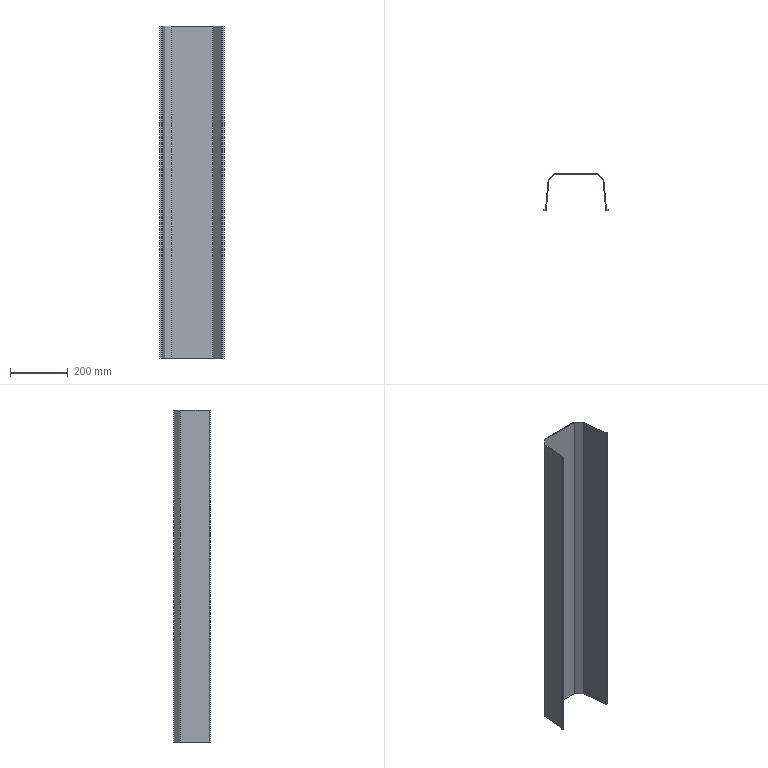Part | STEP file | 51E-01223JG10 | 1 solid | 56 faces | box 225 x 127 x 1150 mm | volume 1231792 mm3 | plane 40 | cylinder 16 | commonest cylinder face diameters 2 x6 7 x6 2.5 x4
STEP:
#1=CARTESIAN_POINT('',(-106.207,0.,575.));
#2=VERTEX_POINT('',#1);
#3=CARTESIAN_POINT('',(-106.207,2.5,575.));
#4=VERTEX_POINT('',#3);
#5=CARTESIAN_POINT('',(-106.207,1.25,575.));
#6=DIRECTION('',(0.,1.,0.));
#7=VECTOR('',#6,1.);
#8=LINE('',#5,#7);
#9=EDGE_CURVE('',#2,#4,#8,.T.);
#10=ORIENTED_EDGE('',*,*,#9,.F.);
#11=CARTESIAN_POINT('',(-102.72,3.195,575.));
#12=VERTEX_POINT('',#11);
#13=CARTESIAN_POINT('',(-102.72,3.195,575.));
#14=CARTESIAN_POINT('',(-102.752,2.83,575.));
#15=CARTESIAN_POINT('',(-102.832,2.469,575.));
#16=CARTESIAN_POINT('',(-102.959,2.12,575.));
#17=CARTESIAN_POINT('',(-103.301,1.465,575.));
#18=CARTESIAN_POINT('',(-103.8,0.9191,575.));
#19=CARTESIAN_POINT('',(-104.084,0.6808,575.));
#20=CARTESIAN_POINT('',(-104.656,0.3172,575.));
#21=CARTESIAN_POINT('',(-105.296,0.09984,575.));
#22=CARTESIAN_POINT('',(-105.597,0.03328,575.));
#23=CARTESIAN_POINT('',(-105.902,0.,575.));
#24=CARTESIAN_POINT('',(-106.207,0.,575.));
#25=B_SPLINE_CURVE_WITH_KNOTS('',5,(#13,#14,#15,#16,#17,#18,#19,#20,#21,#22,#23,#24),.UNSPECIFIED.,.F.,.U.,(6,3,3,6),(0.,2.592,5.185,7.343),.UNSPECIFIED.);
#26=EDGE_CURVE('',#12,#2,#25,.T.);
#27=ORIENTED_EDGE('',*,*,#26,.F.);
#28=CARTESIAN_POINT('',(-105.211,3.413,575.));
#29=VERTEX_POINT('',#28);
#30=CARTESIAN_POINT('',(-103.966,3.304,575.));
#31=DIRECTION('',(0.9962,-0.08716,0.));
#32=VECTOR('',#31,1.);
#33=LINE('',#30,#32);
#34=EDGE_CURVE('',#29,#12,#33,.T.);
#35=ORIENTED_EDGE('',*,*,#34,.F.);
#36=CARTESIAN_POINT('',(-105.211,3.413,575.));
#37=CARTESIAN_POINT('',(-105.22,3.315,575.));
#38=CARTESIAN_POINT('',(-105.24,3.219,575.));
#39=CARTESIAN_POINT('',(-105.272,3.125,575.));
#40=CARTESIAN_POINT('',(-105.359,2.948,575.));
#41=CARTESIAN_POINT('',(-105.486,2.797,575.));
#42=CARTESIAN_POINT('',(-105.559,2.729,575.));
#43=CARTESIAN_POINT('',(-105.719,2.614,575.));
#44=CARTESIAN_POINT('',(-105.902,2.54,575.));
#45=CARTESIAN_POINT('',(-105.998,2.515,575.));
#46=CARTESIAN_POINT('',(-106.098,2.501,575.));
#47=CARTESIAN_POINT('',(-106.199,2.5,575.));
#48=CARTESIAN_POINT('',(-106.202,2.5,575.));
#49=CARTESIAN_POINT('',(-106.204,2.5,575.));
#50=CARTESIAN_POINT('',(-106.207,2.5,575.));
#51=B_SPLINE_CURVE_WITH_KNOTS('',5,(#36,#37,#38,#39,#40,#41,#42,#43,#44,#45,#46,#47,#48,#49,#50),.UNSPECIFIED.,.F.,.U.,(6,3,3,3,6),(0.,0.6928,1.386,2.078,2.098),.UNSPECIFIED.);
#52=EDGE_CURVE('',#29,#4,#51,.T.);
#53=ORIENTED_EDGE('',*,*,#52,.T.);
#54=EDGE_LOOP('',(#10,#27,#35,#53));
#55=FACE_OUTER_BOUND('',#54,.T.);
#56=CARTESIAN_POINT('',(-106.207,0.,575.));
#57=DIRECTION('',(0.,0.,1.));
#58=DIRECTION('',(1.,0.,0.));
#59=AXIS2_PLACEMENT_3D('',#56,#57,#58);
#60=PLANE('',#59);
#61=ADVANCED_FACE('',(#55),#60,.T.);
#62=CARTESIAN_POINT('',(-111.25,2.5,575.));
#63=VERTEX_POINT('',#62);
#64=CARTESIAN_POINT('',(-112.5,1.25,575.));
#65=VERTEX_POINT('',#64);
#66=CARTESIAN_POINT('',(-111.25,1.25,575.));
#67=DIRECTION('',(0.,0.,1.));
#68=AXIS2_PLACEMENT_3D('',#66,#67,$);
#69=CIRCLE('',#68,1.25);
#70=EDGE_CURVE('',#63,#65,#69,.T.);
#71=ORIENTED_EDGE('',*,*,#70,.T.);
#72=CARTESIAN_POINT('',(-111.25,0.,575.));
#73=VERTEX_POINT('',#72);
#74=CARTESIAN_POINT('',(-111.25,1.25,575.));
#75=DIRECTION('',(0.,0.,1.));
#76=AXIS2_PLACEMENT_3D('',#74,#75,$);
#77=CIRCLE('',#76,1.25);
#78=EDGE_CURVE('',#65,#73,#77,.T.);
#79=ORIENTED_EDGE('',*,*,#78,.T.);
#80=CARTESIAN_POINT('',(-108.729,0.,575.));
#81=DIRECTION('',(-1.,0.,0.));
#82=VECTOR('',#81,1.);
#83=LINE('',#80,#82);
#84=EDGE_CURVE('',#2,#73,#83,.T.);
#85=ORIENTED_EDGE('',*,*,#84,.F.);
#86=ORIENTED_EDGE('',*,*,#9,.T.);
#87=CARTESIAN_POINT('',(-108.729,2.5,575.));
#88=DIRECTION('',(-1.,0.,0.));
#89=VECTOR('',#88,1.);
#90=LINE('',#87,#89);
#91=EDGE_CURVE('',#4,#63,#90,.T.);
#92=ORIENTED_EDGE('',*,*,#91,.T.);
#93=EDGE_LOOP('',(#71,#79,#85,#86,#92));
#94=FACE_OUTER_BOUND('',#93,.T.);
#95=CARTESIAN_POINT('',(-105.211,3.413,575.));
#96=DIRECTION('',(0.,0.,1.));
#97=DIRECTION('',(1.,0.,0.));
#98=AXIS2_PLACEMENT_3D('',#95,#96,#97);
#99=PLANE('',#98);
#100=ADVANCED_FACE('',(#94),#99,.T.);
#101=CARTESIAN_POINT('',(-102.72,3.195,-575.));
#102=VERTEX_POINT('',#101);
#103=CARTESIAN_POINT('',(-106.207,0.,-575.));
#104=VERTEX_POINT('',#103);
#105=CARTESIAN_POINT('',(-106.207,3.5,-575.));
#106=DIRECTION('',(0.,0.,-1.));
#107=AXIS2_PLACEMENT_3D('',#105,#106,$);
#108=CIRCLE('',#107,3.5);
#109=EDGE_CURVE('',#102,#104,#108,.T.);
#110=ORIENTED_EDGE('',*,*,#109,.F.);
#111=CARTESIAN_POINT('',(-102.72,3.195,575.));
#112=DIRECTION('',(0.,0.,-1.));
#113=VECTOR('',#112,1.);
#114=LINE('',#111,#113);
#115=EDGE_CURVE('',#12,#102,#114,.T.);
#116=ORIENTED_EDGE('',*,*,#115,.F.);
#117=ORIENTED_EDGE('',*,*,#26,.T.);
#118=CARTESIAN_POINT('',(-106.207,0.,575.));
#119=DIRECTION('',(0.,0.,-1.));
#120=VECTOR('',#119,1.);
#121=LINE('',#118,#120);
#122=EDGE_CURVE('',#2,#104,#121,.T.);
#123=ORIENTED_EDGE('',*,*,#122,.T.);
#124=EDGE_LOOP('',(#110,#116,#117,#123));
#125=FACE_OUTER_BOUND('',#124,.T.);
#126=CARTESIAN_POINT('',(-106.207,3.5,575.));
#127=DIRECTION('',(0.,0.,-1.));
#128=DIRECTION('',(1.,0.,0.));
#129=AXIS2_PLACEMENT_3D('',#126,#127,#128);
#130=CYLINDRICAL_SURFACE('',#129,3.5);
#131=ADVANCED_FACE('',(#125),#130,.T.);
#132=CARTESIAN_POINT('',(-94.02,102.637,575.));
#133=VERTEX_POINT('',#132);
#134=CARTESIAN_POINT('',(-98.37,52.916,575.));
#135=DIRECTION('',(-0.08716,-0.9962,0.));
#136=VECTOR('',#135,1.);
#137=LINE('',#134,#136);
#138=EDGE_CURVE('',#133,#12,#137,.T.);
#139=ORIENTED_EDGE('',*,*,#138,.F.);
#140=CARTESIAN_POINT('',(-96.511,102.855,575.));
#141=VERTEX_POINT('',#140);
#142=CARTESIAN_POINT('',(-95.266,102.746,575.));
#143=DIRECTION('',(-0.9962,0.08716,0.));
#144=VECTOR('',#143,1.);
#145=LINE('',#142,#144);
#146=EDGE_CURVE('',#133,#141,#145,.T.);
#147=ORIENTED_EDGE('',*,*,#146,.T.);
#148=CARTESIAN_POINT('',(-100.861,53.134,575.));
#149=DIRECTION('',(-0.08716,-0.9962,0.));
#150=VECTOR('',#149,1.);
#151=LINE('',#148,#150);
#152=EDGE_CURVE('',#141,#29,#151,.T.);
#153=ORIENTED_EDGE('',*,*,#152,.T.);
#154=ORIENTED_EDGE('',*,*,#34,.T.);
#155=EDGE_LOOP('',(#139,#147,#153,#154));
#156=FACE_OUTER_BOUND('',#155,.T.);
#157=CARTESIAN_POINT('',(-95.499,105.025,575.));
#158=DIRECTION('',(0.,0.,1.));
#159=DIRECTION('',(1.,0.,0.));
#160=AXIS2_PLACEMENT_3D('',#157,#158,#159);
#161=PLANE('',#160);
#162=ADVANCED_FACE('',(#156),#161,.T.);
#163=CARTESIAN_POINT('',(-105.211,3.413,-575.));
#164=VERTEX_POINT('',#163);
#165=CARTESIAN_POINT('',(-106.207,2.5,-575.));
#166=VERTEX_POINT('',#165);
#167=CARTESIAN_POINT('',(-106.207,3.5,-575.));
#168=DIRECTION('',(0.,0.,-1.));
#169=AXIS2_PLACEMENT_3D('',#167,#168,$);
#170=CIRCLE('',#169,1.);
#171=EDGE_CURVE('',#164,#166,#170,.T.);
#172=ORIENTED_EDGE('',*,*,#171,.T.);
#173=CARTESIAN_POINT('',(-106.207,2.5,575.));
#174=DIRECTION('',(0.,0.,-1.));
#175=VECTOR('',#174,1.);
#176=LINE('',#173,#175);
#177=EDGE_CURVE('',#4,#166,#176,.T.);
#178=ORIENTED_EDGE('',*,*,#177,.F.);
#179=ORIENTED_EDGE('',*,*,#52,.F.);
#180=CARTESIAN_POINT('',(-105.211,3.413,575.));
#181=DIRECTION('',(0.,0.,-1.));
#182=VECTOR('',#181,1.);
#183=LINE('',#180,#182);
#184=EDGE_CURVE('',#29,#164,#183,.T.);
#185=ORIENTED_EDGE('',*,*,#184,.T.);
#186=EDGE_LOOP('',(#172,#178,#179,#185));
#187=FACE_OUTER_BOUND('',#186,.T.);
#188=CARTESIAN_POINT('',(-106.207,3.5,575.));
#189=DIRECTION('',(0.,0.,-1.));
#190=DIRECTION('',(1.,0.,0.));
#191=AXIS2_PLACEMENT_3D('',#188,#189,#190);
#192=CYLINDRICAL_SURFACE('',#191,1.);
#193=ADVANCED_FACE('',(#187),#192,.F.);
#194=CARTESIAN_POINT('',(-112.5,1.25,-575.));
#195=VERTEX_POINT('',#194);
#196=CARTESIAN_POINT('',(-112.5,1.25,575.));
#197=DIRECTION('',(0.,0.,1.));
#198=VECTOR('',#197,1.);
#199=LINE('',#196,#198);
#200=EDGE_CURVE('',#65,#195,#199,.F.);
#201=ORIENTED_EDGE('',*,*,#200,.F.);
#202=ORIENTED_EDGE('',*,*,#70,.F.);
#203=CARTESIAN_POINT('',(-111.25,2.5,-575.));
#204=VERTEX_POINT('',#203);
#205=CARTESIAN_POINT('',(-111.25,2.5,575.));
#206=DIRECTION('',(0.,0.,1.));
#207=VECTOR('',#206,1.);
#208=LINE('',#205,#207);
#209=EDGE_CURVE('',#204,#63,#208,.T.);
#210=ORIENTED_EDGE('',*,*,#209,.F.);
#211=CARTESIAN_POINT('',(-111.25,1.25,-575.));
#212=DIRECTION('',(0.,0.,1.));
#213=AXIS2_PLACEMENT_3D('',#211,#212,$);
#214=CIRCLE('',#213,1.25);
#215=EDGE_CURVE('',#195,#204,#214,.F.);
#216=ORIENTED_EDGE('',*,*,#215,.F.);
#217=EDGE_LOOP('',(#201,#202,#210,#216));
#218=FACE_OUTER_BOUND('',#217,.T.);
#219=CARTESIAN_POINT('',(-111.25,1.25,575.));
#220=DIRECTION('',(0.,0.,1.));
#221=DIRECTION('',(1.,0.,0.));
#222=AXIS2_PLACEMENT_3D('',#219,#220,#221);
#223=CYLINDRICAL_SURFACE('',#222,1.25);
#224=ADVANCED_FACE('',(#218),#223,.T.);
#225=ORIENTED_EDGE('',*,*,#78,.F.);
#226=ORIENTED_EDGE('',*,*,#200,.T.);
#227=CARTESIAN_POINT('',(-111.25,0.,-575.));
#228=VERTEX_POINT('',#227);
#229=CARTESIAN_POINT('',(-111.25,1.25,-575.));
#230=DIRECTION('',(0.,0.,-1.));
#231=AXIS2_PLACEMENT_3D('',#229,#230,$);
#232=CIRCLE('',#231,1.25);
#233=EDGE_CURVE('',#228,#195,#232,.T.);
#234=ORIENTED_EDGE('',*,*,#233,.F.);
#235=CARTESIAN_POINT('',(-111.25,0.,575.));
#236=DIRECTION('',(0.,0.,-1.));
#237=VECTOR('',#236,1.);
#238=LINE('',#235,#237);
#239=EDGE_CURVE('',#73,#228,#238,.T.);
#240=ORIENTED_EDGE('',*,*,#239,.F.);
#241=EDGE_LOOP('',(#225,#226,#234,#240));
#242=FACE_OUTER_BOUND('',#241,.T.);
#243=CARTESIAN_POINT('',(-111.25,1.25,575.));
#244=DIRECTION('',(0.,0.,-1.));
#245=DIRECTION('',(1.,0.,0.));
#246=AXIS2_PLACEMENT_3D('',#243,#244,#245);
#247=CYLINDRICAL_SURFACE('',#246,1.25);
#248=ADVANCED_FACE('',(#242),#247,.T.);
#249=ORIENTED_EDGE('',*,*,#84,.T.);
#250=ORIENTED_EDGE('',*,*,#239,.T.);
#251=CARTESIAN_POINT('',(-108.729,0.,-575.));
#252=DIRECTION('',(-1.,0.,0.));
#253=VECTOR('',#252,1.);
#254=LINE('',#251,#253);
#255=EDGE_CURVE('',#104,#228,#254,.T.);
#256=ORIENTED_EDGE('',*,*,#255,.F.);
#257=ORIENTED_EDGE('',*,*,#122,.F.);
#258=EDGE_LOOP('',(#249,#250,#256,#257));
#259=FACE_OUTER_BOUND('',#258,.T.);
#260=CARTESIAN_POINT('',(-112.5,0.,575.));
#261=DIRECTION('',(0.,-1.,0.));
#262=DIRECTION('',(0.,0.,-1.));
#263=AXIS2_PLACEMENT_3D('',#260,#261,#262);
#264=PLANE('',#263);
#265=ADVANCED_FACE('',(#259),#264,.T.);
#266=CARTESIAN_POINT('',(-108.729,2.5,-575.));
#267=DIRECTION('',(-1.,0.,0.));
#268=VECTOR('',#267,1.);
#269=LINE('',#266,#268);
#270=EDGE_CURVE('',#166,#204,#269,.T.);
#271=ORIENTED_EDGE('',*,*,#270,.T.);
#272=ORIENTED_EDGE('',*,*,#209,.T.);
#273=ORIENTED_EDGE('',*,*,#91,.F.);
#274=ORIENTED_EDGE('',*,*,#177,.T.);
#275=EDGE_LOOP('',(#271,#272,#273,#274));
#276=FACE_OUTER_BOUND('',#275,.T.);
#277=CARTESIAN_POINT('',(-112.5,2.5,575.));
#278=DIRECTION('',(0.,-1.,0.));
#279=DIRECTION('',(0.,0.,-1.));
#280=AXIS2_PLACEMENT_3D('',#277,#278,#279);
#281=PLANE('',#280);
#282=ADVANCED_FACE('',(#276),#281,.F.);
#283=CARTESIAN_POINT('',(-103.966,3.304,-575.));
#284=DIRECTION('',(-0.9962,0.08716,0.));
#285=VECTOR('',#284,1.);
#286=LINE('',#283,#285);
#287=EDGE_CURVE('',#102,#164,#286,.T.);
#288=ORIENTED_EDGE('',*,*,#287,.F.);
#289=ORIENTED_EDGE('',*,*,#109,.T.);
#290=CARTESIAN_POINT('',(-106.207,1.25,-575.));
#291=DIRECTION('',(0.,-1.,0.));
#292=VECTOR('',#291,1.);
#293=LINE('',#290,#292);
#294=EDGE_CURVE('',#166,#104,#293,.T.);
#295=ORIENTED_EDGE('',*,*,#294,.F.);
#296=ORIENTED_EDGE('',*,*,#171,.F.);
#297=EDGE_LOOP('',(#288,#289,#295,#296));
#298=FACE_OUTER_BOUND('',#297,.T.);
#299=CARTESIAN_POINT('',(-102.72,3.195,-575.));
#300=DIRECTION('',(0.,0.,-1.));
#301=DIRECTION('',(-1.,0.,0.));
#302=AXIS2_PLACEMENT_3D('',#299,#300,#301);
#303=PLANE('',#302);
#304=ADVANCED_FACE('',(#298),#303,.T.);
#305=CARTESIAN_POINT('',(-94.02,102.637,-575.));
#306=VERTEX_POINT('',#305);
#307=CARTESIAN_POINT('',(-98.37,52.916,-575.));
#308=DIRECTION('',(-0.08716,-0.9962,0.));
#309=VECTOR('',#308,1.);
#310=LINE('',#307,#309);
#311=EDGE_CURVE('',#306,#102,#310,.T.);
#312=ORIENTED_EDGE('',*,*,#311,.F.);
#313=CARTESIAN_POINT('',(-94.02,102.637,0.));
#314=DIRECTION('',(0.,0.,-1.));
#315=VECTOR('',#314,1.);
#316=LINE('',#313,#315);
#317=EDGE_CURVE('',#133,#306,#316,.T.);
#318=ORIENTED_EDGE('',*,*,#317,.F.);
#319=ORIENTED_EDGE('',*,*,#138,.T.);
#320=ORIENTED_EDGE('',*,*,#115,.T.);
#321=EDGE_LOOP('',(#312,#318,#319,#320));
#322=FACE_OUTER_BOUND('',#321,.T.);
#323=CARTESIAN_POINT('',(-103.,0.,575.));
#324=DIRECTION('',(0.9962,-0.08716,0.));
#325=DIRECTION('',(0.08716,0.9962,0.));
#326=AXIS2_PLACEMENT_3D('',#323,#324,#325);
#327=PLANE('',#326);
#328=ADVANCED_FACE('',(#322),#327,.T.);
#329=ORIENTED_EDGE('',*,*,#146,.F.);
#330=CARTESIAN_POINT('',(-93.731,103.257,575.));
#331=VERTEX_POINT('',#330);
#332=CARTESIAN_POINT('',(-93.024,102.55,575.));
#333=DIRECTION('',(0.,0.,1.));
#334=AXIS2_PLACEMENT_3D('',#332,#333,$);
#335=CIRCLE('',#334,1.);
#336=EDGE_CURVE('',#331,#133,#335,.T.);
#337=ORIENTED_EDGE('',*,*,#336,.F.);
#338=CARTESIAN_POINT('',(-95.499,105.025,575.));
#339=VERTEX_POINT('',#338);
#340=CARTESIAN_POINT('',(-94.615,104.141,575.));
#341=DIRECTION('',(0.7071,-0.7071,0.));
#342=VECTOR('',#341,1.);
#343=LINE('',#340,#342);
#344=EDGE_CURVE('',#339,#331,#343,.T.);
#345=ORIENTED_EDGE('',*,*,#344,.F.);
#346=CARTESIAN_POINT('',(-93.024,102.55,575.));
#347=DIRECTION('',(0.,0.,1.));
#348=AXIS2_PLACEMENT_3D('',#346,#347,$);
#349=CIRCLE('',#348,3.5);
#350=EDGE_CURVE('',#339,#141,#349,.T.);
#351=ORIENTED_EDGE('',*,*,#350,.T.);
#352=EDGE_LOOP('',(#329,#337,#345,#351));
#353=FACE_OUTER_BOUND('',#352,.T.);
#354=CARTESIAN_POINT('',(-94.02,102.637,575.));
#355=DIRECTION('',(0.,0.,1.));
#356=DIRECTION('',(1.,0.,0.));
#357=AXIS2_PLACEMENT_3D('',#354,#355,#356);
#358=PLANE('',#357);
#359=ADVANCED_FACE('',(#353),#358,.T.);
#360=CARTESIAN_POINT('',(-96.511,102.855,-575.));
#361=VERTEX_POINT('',#360);
#362=CARTESIAN_POINT('',(-100.861,53.134,-575.));
#363=DIRECTION('',(-0.08716,-0.9962,0.));
#364=VECTOR('',#363,1.);
#365=LINE('',#362,#364);
#366=EDGE_CURVE('',#361,#164,#365,.T.);
#367=ORIENTED_EDGE('',*,*,#366,.T.);
#368=ORIENTED_EDGE('',*,*,#184,.F.);
#369=ORIENTED_EDGE('',*,*,#152,.F.);
#370=CARTESIAN_POINT('',(-96.511,102.855,0.));
#371=DIRECTION('',(0.,0.,-1.));
#372=VECTOR('',#371,1.);
#373=LINE('',#370,#372);
#374=EDGE_CURVE('',#141,#361,#373,.T.);
#375=ORIENTED_EDGE('',*,*,#374,.T.);
#376=EDGE_LOOP('',(#367,#368,#369,#375));
#377=FACE_OUTER_BOUND('',#376,.T.);
#378=CARTESIAN_POINT('',(-105.49,0.2179,575.));
#379=DIRECTION('',(0.9962,-0.08716,0.));
#380=DIRECTION('',(0.08716,0.9962,0.));
#381=AXIS2_PLACEMENT_3D('',#378,#379,#380);
#382=PLANE('',#381);
#383=ADVANCED_FACE('',(#377),#382,.F.);
#384=ORIENTED_EDGE('',*,*,#255,.T.);
#385=ORIENTED_EDGE('',*,*,#233,.T.);
#386=ORIENTED_EDGE('',*,*,#215,.T.);
#387=ORIENTED_EDGE('',*,*,#270,.F.);
#388=ORIENTED_EDGE('',*,*,#294,.T.);
#389=EDGE_LOOP('',(#384,#385,#386,#387,#388));
#390=FACE_OUTER_BOUND('',#389,.T.);
#391=CARTESIAN_POINT('',(-106.207,3.5,-575.));
#392=DIRECTION('',(0.,0.,-1.));
#393=DIRECTION('',(-1.,0.,0.));
#394=AXIS2_PLACEMENT_3D('',#391,#392,#393);
#395=PLANE('',#394);
#396=ADVANCED_FACE('',(#390),#395,.T.);
#397=ORIENTED_EDGE('',*,*,#311,.T.);
#398=ORIENTED_EDGE('',*,*,#287,.T.);
#399=ORIENTED_EDGE('',*,*,#366,.F.);
#400=CARTESIAN_POINT('',(-95.266,102.746,-575.));
#401=DIRECTION('',(0.9962,-0.08716,0.));
#402=VECTOR('',#401,1.);
#403=LINE('',#400,#402);
#404=EDGE_CURVE('',#361,#306,#403,.T.);
#405=ORIENTED_EDGE('',*,*,#404,.T.);
#406=EDGE_LOOP('',(#397,#398,#399,#405));
#407=FACE_OUTER_BOUND('',#406,.T.);
#408=CARTESIAN_POINT('',(-106.207,2.5,-575.));
#409=DIRECTION('',(0.,0.,-1.));
#410=DIRECTION('',(-1.,0.,0.));
#411=AXIS2_PLACEMENT_3D('',#408,#409,#410);
#412=PLANE('',#411);
#413=ADVANCED_FACE('',(#407),#412,.T.);
#414=CARTESIAN_POINT('',(-93.731,103.257,-575.));
#415=VERTEX_POINT('',#414);
#416=CARTESIAN_POINT('',(-93.024,102.55,-575.));
#417=DIRECTION('',(0.,0.,-1.));
#418=AXIS2_PLACEMENT_3D('',#416,#417,$);
#419=CIRCLE('',#418,1.);
#420=EDGE_CURVE('',#415,#306,#419,.F.);
#421=ORIENTED_EDGE('',*,*,#420,.F.);
#422=CARTESIAN_POINT('',(-93.731,103.257,575.));
#423=DIRECTION('',(0.,0.,-1.));
#424=VECTOR('',#423,1.);
#425=LINE('',#422,#424);
#426=EDGE_CURVE('',#331,#415,#425,.T.);
#427=ORIENTED_EDGE('',*,*,#426,.F.);
#428=ORIENTED_EDGE('',*,*,#336,.T.);
#429=ORIENTED_EDGE('',*,*,#317,.T.);
#430=EDGE_LOOP('',(#421,#427,#428,#429));
#431=FACE_OUTER_BOUND('',#430,.T.);
#432=CARTESIAN_POINT('',(-93.024,102.55,575.));
#433=DIRECTION('',(0.,0.,-1.));
#434=DIRECTION('',(-1.,0.,0.));
#435=AXIS2_PLACEMENT_3D('',#432,#433,#434);
#436=CYLINDRICAL_SURFACE('',#435,1.);
#437=ADVANCED_FACE('',(#431),#436,.F.);
#438=CARTESIAN_POINT('',(-72.782,124.207,575.));
#439=VERTEX_POINT('',#438);
#440=CARTESIAN_POINT('',(-83.256,113.732,575.));
#441=DIRECTION('',(-0.7071,-0.7071,0.));
#442=VECTOR('',#441,1.);
#443=LINE('',#440,#442);
#444=EDGE_CURVE('',#439,#331,#443,.T.);
#445=ORIENTED_EDGE('',*,*,#444,.F.);
#446=CARTESIAN_POINT('',(-74.549,125.975,575.));
#447=VERTEX_POINT('',#446);
#448=CARTESIAN_POINT('',(-73.665,125.091,575.));
#449=DIRECTION('',(-0.7071,0.7071,0.));
#450=VECTOR('',#449,1.);
#451=LINE('',#448,#450);
#452=EDGE_CURVE('',#439,#447,#451,.T.);
#453=ORIENTED_EDGE('',*,*,#452,.T.);
#454=CARTESIAN_POINT('',(-85.024,115.5,575.));
#455=DIRECTION('',(-0.7071,-0.7071,0.));
#456=VECTOR('',#455,1.);
#457=LINE('',#454,#456);
#458=EDGE_CURVE('',#447,#339,#457,.T.);
#459=ORIENTED_EDGE('',*,*,#458,.T.);
#460=ORIENTED_EDGE('',*,*,#344,.T.);
#461=EDGE_LOOP('',(#445,#453,#459,#460));
#462=FACE_OUTER_BOUND('',#461,.T.);
#463=CARTESIAN_POINT('',(-72.074,127.,575.));
#464=DIRECTION('',(0.,0.,1.));
#465=DIRECTION('',(1.,0.,0.));
#466=AXIS2_PLACEMENT_3D('',#463,#464,#465);
#467=PLANE('',#466);
#468=ADVANCED_FACE('',(#462),#467,.T.);
#469=CARTESIAN_POINT('',(-95.499,105.025,-575.));
#470=VERTEX_POINT('',#469);
#471=CARTESIAN_POINT('',(-93.024,102.55,-575.));
#472=DIRECTION('',(0.,0.,-1.));
#473=AXIS2_PLACEMENT_3D('',#471,#472,$);
#474=CIRCLE('',#473,3.5);
#475=EDGE_CURVE('',#470,#361,#474,.F.);
#476=ORIENTED_EDGE('',*,*,#475,.T.);
#477=ORIENTED_EDGE('',*,*,#374,.F.);
#478=ORIENTED_EDGE('',*,*,#350,.F.);
#479=CARTESIAN_POINT('',(-95.499,105.025,575.));
#480=DIRECTION('',(0.,0.,-1.));
#481=VECTOR('',#480,1.);
#482=LINE('',#479,#481);
#483=EDGE_CURVE('',#339,#470,#482,.T.);
#484=ORIENTED_EDGE('',*,*,#483,.T.);
#485=EDGE_LOOP('',(#476,#477,#478,#484));
#486=FACE_OUTER_BOUND('',#485,.T.);
#487=CARTESIAN_POINT('',(-93.024,102.55,575.));
#488=DIRECTION('',(0.,0.,-1.));
#489=DIRECTION('',(-1.,0.,0.));
#490=AXIS2_PLACEMENT_3D('',#487,#488,#489);
#491=CYLINDRICAL_SURFACE('',#490,3.5);
#492=ADVANCED_FACE('',(#486),#491,.T.);
#493=CARTESIAN_POINT('',(-94.615,104.141,-575.));
#494=DIRECTION('',(-0.7071,0.7071,0.));
#495=VECTOR('',#494,1.);
#496=LINE('',#493,#495);
#497=EDGE_CURVE('',#415,#470,#496,.T.);
#498=ORIENTED_EDGE('',*,*,#497,.F.);
#499=ORIENTED_EDGE('',*,*,#420,.T.);
#500=ORIENTED_EDGE('',*,*,#404,.F.);
#501=ORIENTED_EDGE('',*,*,#475,.F.);
#502=EDGE_LOOP('',(#498,#499,#500,#501));
#503=FACE_OUTER_BOUND('',#502,.T.);
#504=CARTESIAN_POINT('',(-93.731,103.257,-575.));
#505=DIRECTION('',(0.,0.,-1.));
#506=DIRECTION('',(-1.,0.,0.));
#507=AXIS2_PLACEMENT_3D('',#504,#505,#506);
#508=PLANE('',#507);
#509=ADVANCED_FACE('',(#503),#508,.T.);
#510=CARTESIAN_POINT('',(-72.782,124.207,-575.));
#511=VERTEX_POINT('',#510);
#512=CARTESIAN_POINT('',(-83.256,113.732,-575.));
#513=DIRECTION('',(-0.7071,-0.7071,0.));
#514=VECTOR('',#513,1.);
#515=LINE('',#512,#514);
#516=EDGE_CURVE('',#511,#415,#515,.T.);
#517=ORIENTED_EDGE('',*,*,#516,.F.);
#518=CARTESIAN_POINT('',(-72.782,124.207,0.));
#519=DIRECTION('',(0.,0.,-1.));
#520=VECTOR('',#519,1.);
#521=LINE('',#518,#520);
#522=EDGE_CURVE('',#439,#511,#521,.T.);
#523=ORIENTED_EDGE('',*,*,#522,.F.);
#524=ORIENTED_EDGE('',*,*,#444,.T.);
#525=ORIENTED_EDGE('',*,*,#426,.T.);
#526=EDGE_LOOP('',(#517,#523,#524,#525));
#527=FACE_OUTER_BOUND('',#526,.T.);
#528=CARTESIAN_POINT('',(-93.989,103.,575.));
#529=DIRECTION('',(0.7071,-0.7071,0.));
#530=DIRECTION('',(0.7071,0.7071,0.));
#531=AXIS2_PLACEMENT_3D('',#528,#529,#530);
#532=PLANE('',#531);
#533=ADVANCED_FACE('',(#527),#532,.T.);
#534=ORIENTED_EDGE('',*,*,#452,.F.);
#535=CARTESIAN_POINT('',(-72.074,124.5,575.));
#536=VERTEX_POINT('',#535);
#537=CARTESIAN_POINT('',(-72.074,123.5,575.));
#538=DIRECTION('',(0.,0.,1.));
#539=AXIS2_PLACEMENT_3D('',#537,#538,$);
#540=CIRCLE('',#539,1.);
#541=EDGE_CURVE('',#536,#439,#540,.T.);
#542=ORIENTED_EDGE('',*,*,#541,.F.);
#543=CARTESIAN_POINT('',(-72.074,127.,575.));
#544=VERTEX_POINT('',#543);
#545=CARTESIAN_POINT('',(-72.074,125.75,575.));
#546=DIRECTION('',(0.,-1.,0.));
#547=VECTOR('',#546,1.);
#548=LINE('',#545,#547);
#549=EDGE_CURVE('',#544,#536,#548,.T.);
#550=ORIENTED_EDGE('',*,*,#549,.F.);
#551=CARTESIAN_POINT('',(-72.074,123.5,575.));
#552=DIRECTION('',(0.,0.,1.));
#553=AXIS2_PLACEMENT_3D('',#551,#552,$);
#554=CIRCLE('',#553,3.5);
#555=EDGE_CURVE('',#544,#447,#554,.T.);
#556=ORIENTED_EDGE('',*,*,#555,.T.);
#557=EDGE_LOOP('',(#534,#542,#550,#556));
#558=FACE_OUTER_BOUND('',#557,.T.);
#559=CARTESIAN_POINT('',(-72.782,124.207,575.));
#560=DIRECTION('',(0.,0.,1.));
#561=DIRECTION('',(1.,0.,0.));
#562=AXIS2_PLACEMENT_3D('',#559,#560,#561);
#563=PLANE('',#562);
#564=ADVANCED_FACE('',(#558),#563,.T.);
#565=CARTESIAN_POINT('',(-74.549,125.975,-575.));
#566=VERTEX_POINT('',#565);
#567=CARTESIAN_POINT('',(-85.024,115.5,-575.));
#568=DIRECTION('',(-0.7071,-0.7071,0.));
#569=VECTOR('',#568,1.);
#570=LINE('',#567,#569);
#571=EDGE_CURVE('',#566,#470,#570,.T.);
#572=ORIENTED_EDGE('',*,*,#571,.T.);
#573=ORIENTED_EDGE('',*,*,#483,.F.);
#574=ORIENTED_EDGE('',*,*,#458,.F.);
#575=CARTESIAN_POINT('',(-74.549,125.975,0.));
#576=DIRECTION('',(0.,0.,-1.));
#577=VECTOR('',#576,1.);
#578=LINE('',#575,#577);
#579=EDGE_CURVE('',#447,#566,#578,.T.);
#580=ORIENTED_EDGE('',*,*,#579,.T.);
#581=EDGE_LOOP('',(#572,#573,#574,#580));
#582=FACE_OUTER_BOUND('',#581,.T.);
#583=CARTESIAN_POINT('',(-95.756,104.768,575.));
#584=DIRECTION('',(0.7071,-0.7071,0.));
#585=DIRECTION('',(0.7071,0.7071,0.));
#586=AXIS2_PLACEMENT_3D('',#583,#584,#585);
#587=PLANE('',#586);
#588=ADVANCED_FACE('',(#582),#587,.F.);
#589=ORIENTED_EDGE('',*,*,#516,.T.);
#590=ORIENTED_EDGE('',*,*,#497,.T.);
#591=ORIENTED_EDGE('',*,*,#571,.F.);
#592=CARTESIAN_POINT('',(-73.665,125.091,-575.));
#593=DIRECTION('',(0.7071,-0.7071,0.));
#594=VECTOR('',#593,1.);
#595=LINE('',#592,#594);
#596=EDGE_CURVE('',#566,#511,#595,.T.);
#597=ORIENTED_EDGE('',*,*,#596,.T.);
#598=EDGE_LOOP('',(#589,#590,#591,#597));
#599=FACE_OUTER_BOUND('',#598,.T.);
#600=CARTESIAN_POINT('',(-96.511,102.855,-575.));
#601=DIRECTION('',(0.,0.,-1.));
#602=DIRECTION('',(-1.,0.,0.));
#603=AXIS2_PLACEMENT_3D('',#600,#601,#602);
#604=PLANE('',#603);
#605=ADVANCED_FACE('',(#599),#604,.T.);
#606=CARTESIAN_POINT('',(-72.074,124.5,-575.));
#607=VERTEX_POINT('',#606);
#608=CARTESIAN_POINT('',(-72.074,123.5,-575.));
#609=DIRECTION('',(0.,0.,-1.));
#610=AXIS2_PLACEMENT_3D('',#608,#609,$);
#611=CIRCLE('',#610,1.);
#612=EDGE_CURVE('',#607,#511,#611,.F.);
#613=ORIENTED_EDGE('',*,*,#612,.F.);
#614=CARTESIAN_POINT('',(-72.074,124.5,575.));
#615=DIRECTION('',(0.,0.,-1.));
#616=VECTOR('',#615,1.);
#617=LINE('',#614,#616);
#618=EDGE_CURVE('',#536,#607,#617,.T.);
#619=ORIENTED_EDGE('',*,*,#618,.F.);
#620=ORIENTED_EDGE('',*,*,#541,.T.);
#621=ORIENTED_EDGE('',*,*,#522,.T.);
#622=EDGE_LOOP('',(#613,#619,#620,#621));
#623=FACE_OUTER_BOUND('',#622,.T.);
#624=CARTESIAN_POINT('',(-72.074,123.5,575.));
#625=DIRECTION('',(0.,0.,-1.));
#626=DIRECTION('',(-1.,0.,0.));
#627=AXIS2_PLACEMENT_3D('',#624,#625,#626);
#628=CYLINDRICAL_SURFACE('',#627,1.);
#629=ADVANCED_FACE('',(#623),#628,.F.);
#630=CARTESIAN_POINT('',(72.074,124.5,575.));
#631=VERTEX_POINT('',#630);
#632=CARTESIAN_POINT('',(0.,124.5,575.));
#633=DIRECTION('',(-1.,0.,0.));
#634=VECTOR('',#633,1.);
#635=LINE('',#632,#634);
#636=EDGE_CURVE('',#631,#536,#635,.T.);
#637=ORIENTED_EDGE('',*,*,#636,.F.);
#638=CARTESIAN_POINT('',(72.074,127.,575.));
#639=VERTEX_POINT('',#638);
#640=CARTESIAN_POINT('',(72.074,125.75,575.));
#641=DIRECTION('',(0.,1.,0.));
#642=VECTOR('',#641,1.);
#643=LINE('',#640,#642);
#644=EDGE_CURVE('',#631,#639,#643,.T.);
#645=ORIENTED_EDGE('',*,*,#644,.T.);
#646=CARTESIAN_POINT('',(0.,127.,575.));
#647=DIRECTION('',(-1.,0.,0.));
#648=VECTOR('',#647,1.);
#649=LINE('',#646,#648);
#650=EDGE_CURVE('',#639,#544,#649,.T.);
#651=ORIENTED_EDGE('',*,*,#650,.T.);
#652=ORIENTED_EDGE('',*,*,#549,.T.);
#653=EDGE_LOOP('',(#637,#645,#651,#652));
#654=FACE_OUTER_BOUND('',#653,.T.);
#655=CARTESIAN_POINT('',(74.549,125.975,575.));
#656=DIRECTION('',(0.,0.,1.));
#657=DIRECTION('',(1.,0.,0.));
#658=AXIS2_PLACEMENT_3D('',#655,#656,#657);
#659=PLANE('',#658);
#660=ADVANCED_FACE('',(#654),#659,.T.);
#661=CARTESIAN_POINT('',(-72.074,127.,-575.));
#662=VERTEX_POINT('',#661);
#663=CARTESIAN_POINT('',(-72.074,123.5,-575.));
#664=DIRECTION('',(0.,0.,-1.));
#665=AXIS2_PLACEMENT_3D('',#663,#664,$);
#666=CIRCLE('',#665,3.5);
#667=EDGE_CURVE('',#662,#566,#666,.F.);
#668=ORIENTED_EDGE('',*,*,#667,.T.);
#669=ORIENTED_EDGE('',*,*,#579,.F.);
#670=ORIENTED_EDGE('',*,*,#555,.F.);
#671=CARTESIAN_POINT('',(-72.074,127.,575.));
#672=DIRECTION('',(0.,0.,-1.));
#673=VECTOR('',#672,1.);
#674=LINE('',#671,#673);
#675=EDGE_CURVE('',#544,#662,#674,.T.);
#676=ORIENTED_EDGE('',*,*,#675,.T.);
#677=EDGE_LOOP('',(#668,#669,#670,#676));
#678=FACE_OUTER_BOUND('',#677,.T.);
#679=CARTESIAN_POINT('',(-72.074,123.5,575.));
#680=DIRECTION('',(0.,0.,-1.));
#681=DIRECTION('',(-1.,0.,0.));
#682=AXIS2_PLACEMENT_3D('',#679,#680,#681);
#683=CYLINDRICAL_SURFACE('',#682,3.5);
#684=ADVANCED_FACE('',(#678),#683,.T.);
#685=CARTESIAN_POINT('',(-72.074,125.75,-575.));
#686=DIRECTION('',(0.,1.,0.));
#687=VECTOR('',#686,1.);
#688=LINE('',#685,#687);
#689=EDGE_CURVE('',#607,#662,#688,.T.);
#690=ORIENTED_EDGE('',*,*,#689,.F.);
#691=ORIENTED_EDGE('',*,*,#612,.T.);
#692=ORIENTED_EDGE('',*,*,#596,.F.);
#693=ORIENTED_EDGE('',*,*,#667,.F.);
#694=EDGE_LOOP('',(#690,#691,#692,#693));
#695=FACE_OUTER_BOUND('',#694,.T.);
#696=CARTESIAN_POINT('',(-72.074,124.5,-575.));
#697=DIRECTION('',(0.,0.,-1.));
#698=DIRECTION('',(-1.,0.,0.));
#699=AXIS2_PLACEMENT_3D('',#696,#697,#698);
#700=PLANE('',#699);
#701=ADVANCED_FACE('',(#695),#700,.T.);
#702=CARTESIAN_POINT('',(72.074,124.5,-575.));
#703=VERTEX_POINT('',#702);
#704=CARTESIAN_POINT('',(0.,124.5,-575.));
#705=DIRECTION('',(-1.,0.,0.));
#706=VECTOR('',#705,1.);
#707=LINE('',#704,#706);
#708=EDGE_CURVE('',#703,#607,#707,.T.);
#709=ORIENTED_EDGE('',*,*,#708,.F.);
#710=CARTESIAN_POINT('',(72.074,124.5,0.));
#711=DIRECTION('',(0.,0.,-1.));
#712=VECTOR('',#711,1.);
#713=LINE('',#710,#712);
#714=EDGE_CURVE('',#631,#703,#713,.T.);
#715=ORIENTED_EDGE('',*,*,#714,.F.);
#716=ORIENTED_EDGE('',*,*,#636,.T.);
#717=ORIENTED_EDGE('',*,*,#618,.T.);
#718=EDGE_LOOP('',(#709,#715,#716,#717));
#719=FACE_OUTER_BOUND('',#718,.T.);
#720=CARTESIAN_POINT('',(-72.489,124.5,575.));
#721=DIRECTION('',(0.,-1.,0.));
#722=DIRECTION('',(0.,0.,-1.));
#723=AXIS2_PLACEMENT_3D('',#720,#721,#722);
#724=PLANE('',#723);
#725=ADVANCED_FACE('',(#719),#724,.T.);
#726=ORIENTED_EDGE('',*,*,#644,.F.);
#727=CARTESIAN_POINT('',(72.782,124.207,575.));
#728=VERTEX_POINT('',#727);
#729=CARTESIAN_POINT('',(72.074,123.5,575.));
#730=DIRECTION('',(0.,0.,1.));
#731=AXIS2_PLACEMENT_3D('',#729,#730,$);
#732=CIRCLE('',#731,1.);
#733=EDGE_CURVE('',#728,#631,#732,.T.);
#734=ORIENTED_EDGE('',*,*,#733,.F.);
#735=CARTESIAN_POINT('',(74.549,125.975,575.));
#736=VERTEX_POINT('',#735);
#737=CARTESIAN_POINT('',(73.665,125.091,575.));
#738=DIRECTION('',(-0.7071,-0.7071,0.));
#739=VECTOR('',#738,1.);
#740=LINE('',#737,#739);
#741=EDGE_CURVE('',#736,#728,#740,.T.);
#742=ORIENTED_EDGE('',*,*,#741,.F.);
#743=CARTESIAN_POINT('',(72.074,123.5,575.));
#744=DIRECTION('',(0.,0.,1.));
#745=AXIS2_PLACEMENT_3D('',#743,#744,$);
#746=CIRCLE('',#745,3.5);
#747=EDGE_CURVE('',#736,#639,#746,.T.);
#748=ORIENTED_EDGE('',*,*,#747,.T.);
#749=EDGE_LOOP('',(#726,#734,#742,#748));
#750=FACE_OUTER_BOUND('',#749,.T.);
#751=CARTESIAN_POINT('',(72.074,124.5,575.));
#752=DIRECTION('',(0.,0.,1.));
#753=DIRECTION('',(1.,0.,0.));
#754=AXIS2_PLACEMENT_3D('',#751,#752,#753);
#755=PLANE('',#754);
#756=ADVANCED_FACE('',(#750),#755,.T.);
#757=CARTESIAN_POINT('',(72.074,127.,-575.));
#758=VERTEX_POINT('',#757);
#759=CARTESIAN_POINT('',(0.,127.,-575.));
#760=DIRECTION('',(-1.,0.,0.));
#761=VECTOR('',#760,1.);
#762=LINE('',#759,#761);
#763=EDGE_CURVE('',#758,#662,#762,.T.);
#764=ORIENTED_EDGE('',*,*,#763,.T.);
#765=ORIENTED_EDGE('',*,*,#675,.F.);
#766=ORIENTED_EDGE('',*,*,#650,.F.);
#767=CARTESIAN_POINT('',(72.074,127.,0.));
#768=DIRECTION('',(0.,0.,-1.));
#769=VECTOR('',#768,1.);
#770=LINE('',#767,#769);
#771=EDGE_CURVE('',#639,#758,#770,.T.);
#772=ORIENTED_EDGE('',*,*,#771,.T.);
#773=EDGE_LOOP('',(#764,#765,#766,#772));
#774=FACE_OUTER_BOUND('',#773,.T.);
#775=CARTESIAN_POINT('',(-72.489,127.,575.));
#776=DIRECTION('',(0.,-1.,0.));
#777=DIRECTION('',(0.,0.,-1.));
#778=AXIS2_PLACEMENT_3D('',#775,#776,#777);
#779=PLANE('',#778);
#780=ADVANCED_FACE('',(#774),#779,.F.);
#781=ORIENTED_EDGE('',*,*,#708,.T.);
#782=ORIENTED_EDGE('',*,*,#689,.T.);
#783=ORIENTED_EDGE('',*,*,#763,.F.);
#784=CARTESIAN_POINT('',(72.074,125.75,-575.));
#785=DIRECTION('',(0.,-1.,0.));
#786=VECTOR('',#785,1.);
#787=LINE('',#784,#786);
#788=EDGE_CURVE('',#758,#703,#787,.T.);
#789=ORIENTED_EDGE('',*,*,#788,.T.);
#790=EDGE_LOOP('',(#781,#782,#783,#789));
#791=FACE_OUTER_BOUND('',#790,.T.);
#792=CARTESIAN_POINT('',(-74.549,125.975,-575.));
#793=DIRECTION('',(0.,0.,-1.));
#794=DIRECTION('',(-1.,0.,0.));
#795=AXIS2_PLACEMENT_3D('',#792,#793,#794);
#796=PLANE('',#795);
#797=ADVANCED_FACE('',(#791),#796,.T.);
#798=CARTESIAN_POINT('',(72.782,124.207,-575.));
#799=VERTEX_POINT('',#798);
#800=CARTESIAN_POINT('',(72.074,123.5,-575.));
#801=DIRECTION('',(0.,0.,-1.));
#802=AXIS2_PLACEMENT_3D('',#800,#801,$);
#803=CIRCLE('',#802,1.);
#804=EDGE_CURVE('',#799,#703,#803,.F.);
#805=ORIENTED_EDGE('',*,*,#804,.F.);
#806=CARTESIAN_POINT('',(72.782,124.207,575.));
#807=DIRECTION('',(0.,0.,-1.));
#808=VECTOR('',#807,1.);
#809=LINE('',#806,#808);
#810=EDGE_CURVE('',#728,#799,#809,.T.);
#811=ORIENTED_EDGE('',*,*,#810,.F.);
#812=ORIENTED_EDGE('',*,*,#733,.T.);
#813=ORIENTED_EDGE('',*,*,#714,.T.);
#814=EDGE_LOOP('',(#805,#811,#812,#813));
#815=FACE_OUTER_BOUND('',#814,.T.);
#816=CARTESIAN_POINT('',(72.074,123.5,575.));
#817=DIRECTION('',(0.,0.,-1.));
#818=DIRECTION('',(-1.,0.,0.));
#819=AXIS2_PLACEMENT_3D('',#816,#817,#818);
#820=CYLINDRICAL_SURFACE('',#819,1.);
#821=ADVANCED_FACE('',(#815),#820,.F.);
#822=CARTESIAN_POINT('',(93.731,103.257,575.));
#823=VERTEX_POINT('',#822);
#824=CARTESIAN_POINT('',(83.256,113.732,575.));
#825=DIRECTION('',(-0.7071,0.7071,0.));
#826=VECTOR('',#825,1.);
#827=LINE('',#824,#826);
#828=EDGE_CURVE('',#823,#728,#827,.T.);
#829=ORIENTED_EDGE('',*,*,#828,.F.);
#830=CARTESIAN_POINT('',(95.499,105.025,575.));
#831=VERTEX_POINT('',#830);
#832=CARTESIAN_POINT('',(94.615,104.141,575.));
#833=DIRECTION('',(0.7071,0.7071,0.));
#834=VECTOR('',#833,1.);
#835=LINE('',#832,#834);
#836=EDGE_CURVE('',#823,#831,#835,.T.);
#837=ORIENTED_EDGE('',*,*,#836,.T.);
#838=CARTESIAN_POINT('',(85.024,115.5,575.));
#839=DIRECTION('',(-0.7071,0.7071,0.));
#840=VECTOR('',#839,1.);
#841=LINE('',#838,#840);
#842=EDGE_CURVE('',#831,#736,#841,.T.);
#843=ORIENTED_EDGE('',*,*,#842,.T.);
#844=ORIENTED_EDGE('',*,*,#741,.T.);
#845=EDGE_LOOP('',(#829,#837,#843,#844));
#846=FACE_OUTER_BOUND('',#845,.T.);
#847=CARTESIAN_POINT('',(96.511,102.855,575.));
#848=DIRECTION('',(0.,0.,1.));
#849=DIRECTION('',(1.,0.,0.));
#850=AXIS2_PLACEMENT_3D('',#847,#848,#849);
#851=PLANE('',#850);
#852=ADVANCED_FACE('',(#846),#851,.T.);
#853=CARTESIAN_POINT('',(74.549,125.975,-575.));
#854=VERTEX_POINT('',#853);
#855=CARTESIAN_POINT('',(72.074,123.5,-575.));
#856=DIRECTION('',(0.,0.,-1.));
#857=AXIS2_PLACEMENT_3D('',#855,#856,$);
#858=CIRCLE('',#857,3.5);
#859=EDGE_CURVE('',#854,#758,#858,.F.);
#860=ORIENTED_EDGE('',*,*,#859,.T.);
#861=ORIENTED_EDGE('',*,*,#771,.F.);
#862=ORIENTED_EDGE('',*,*,#747,.F.);
#863=CARTESIAN_POINT('',(74.549,125.975,575.));
#864=DIRECTION('',(0.,0.,-1.));
#865=VECTOR('',#864,1.);
#866=LINE('',#863,#865);
#867=EDGE_CURVE('',#736,#854,#866,.T.);
#868=ORIENTED_EDGE('',*,*,#867,.T.);
#869=EDGE_LOOP('',(#860,#861,#862,#868));
#870=FACE_OUTER_BOUND('',#869,.T.);
#871=CARTESIAN_POINT('',(72.074,123.5,575.));
#872=DIRECTION('',(0.,0.,-1.));
#873=DIRECTION('',(-1.,0.,0.));
#874=AXIS2_PLACEMENT_3D('',#871,#872,#873);
#875=CYLINDRICAL_SURFACE('',#874,3.5);
#876=ADVANCED_FACE('',(#870),#875,.T.);
#877=CARTESIAN_POINT('',(73.665,125.091,-575.));
#878=DIRECTION('',(0.7071,0.7071,0.));
#879=VECTOR('',#878,1.);
#880=LINE('',#877,#879);
#881=EDGE_CURVE('',#799,#854,#880,.T.);
#882=ORIENTED_EDGE('',*,*,#881,.F.);
#883=ORIENTED_EDGE('',*,*,#804,.T.);
#884=ORIENTED_EDGE('',*,*,#788,.F.);
#885=ORIENTED_EDGE('',*,*,#859,.F.);
#886=EDGE_LOOP('',(#882,#883,#884,#885));
#887=FACE_OUTER_BOUND('',#886,.T.);
#888=CARTESIAN_POINT('',(72.782,124.207,-575.));
#889=DIRECTION('',(0.,0.,-1.));
#890=DIRECTION('',(-1.,0.,0.));
#891=AXIS2_PLACEMENT_3D('',#888,#889,#890);
#892=PLANE('',#891);
#893=ADVANCED_FACE('',(#887),#892,.T.);
#894=CARTESIAN_POINT('',(93.731,103.257,-575.));
#895=VERTEX_POINT('',#894);
#896=CARTESIAN_POINT('',(83.256,113.732,-575.));
#897=DIRECTION('',(-0.7071,0.7071,0.));
#898=VECTOR('',#897,1.);
#899=LINE('',#896,#898);
#900=EDGE_CURVE('',#895,#799,#899,.T.);
#901=ORIENTED_EDGE('',*,*,#900,.F.);
#902=CARTESIAN_POINT('',(93.731,103.257,0.));
#903=DIRECTION('',(0.,0.,-1.));
#904=VECTOR('',#903,1.);
#905=LINE('',#902,#904);
#906=EDGE_CURVE('',#823,#895,#905,.T.);
#907=ORIENTED_EDGE('',*,*,#906,.F.);
#908=ORIENTED_EDGE('',*,*,#828,.T.);
#909=ORIENTED_EDGE('',*,*,#810,.T.);
#910=EDGE_LOOP('',(#901,#907,#908,#909));
#911=FACE_OUTER_BOUND('',#910,.T.);
#912=CARTESIAN_POINT('',(93.989,103.,575.));
#913=DIRECTION('',(-0.7071,-0.7071,0.));
#914=DIRECTION('',(0.7071,-0.7071,0.));
#915=AXIS2_PLACEMENT_3D('',#912,#913,#914);
#916=PLANE('',#915);
#917=ADVANCED_FACE('',(#911),#916,.T.);
#918=ORIENTED_EDGE('',*,*,#836,.F.);
#919=CARTESIAN_POINT('',(94.02,102.637,575.));
#920=VERTEX_POINT('',#919);
#921=CARTESIAN_POINT('',(93.024,102.55,575.));
#922=DIRECTION('',(0.,0.,1.));
#923=AXIS2_PLACEMENT_3D('',#921,#922,$);
#924=CIRCLE('',#923,1.);
#925=EDGE_CURVE('',#920,#823,#924,.T.);
#926=ORIENTED_EDGE('',*,*,#925,.F.);
#927=CARTESIAN_POINT('',(96.511,102.855,575.));
#928=VERTEX_POINT('',#927);
#929=CARTESIAN_POINT('',(95.266,102.746,575.));
#930=DIRECTION('',(-0.9962,-0.08716,0.));
#931=VECTOR('',#930,1.);
#932=LINE('',#929,#931);
#933=EDGE_CURVE('',#928,#920,#932,.T.);
#934=ORIENTED_EDGE('',*,*,#933,.F.);
#935=CARTESIAN_POINT('',(93.024,102.55,575.));
#936=DIRECTION('',(0.,0.,1.));
#937=AXIS2_PLACEMENT_3D('',#935,#936,$);
#938=CIRCLE('',#937,3.5);
#939=EDGE_CURVE('',#928,#831,#938,.T.);
#940=ORIENTED_EDGE('',*,*,#939,.T.);
#941=EDGE_LOOP('',(#918,#926,#934,#940));
#942=FACE_OUTER_BOUND('',#941,.T.);
#943=CARTESIAN_POINT('',(93.731,103.257,575.));
#944=DIRECTION('',(0.,0.,1.));
#945=DIRECTION('',(1.,0.,0.));
#946=AXIS2_PLACEMENT_3D('',#943,#944,#945);
#947=PLANE('',#946);
#948=ADVANCED_FACE('',(#942),#947,.T.);
#949=CARTESIAN_POINT('',(95.499,105.025,-575.));
#950=VERTEX_POINT('',#949);
#951=CARTESIAN_POINT('',(85.024,115.5,-575.));
#952=DIRECTION('',(-0.7071,0.7071,0.));
#953=VECTOR('',#952,1.);
#954=LINE('',#951,#953);
#955=EDGE_CURVE('',#950,#854,#954,.T.);
#956=ORIENTED_EDGE('',*,*,#955,.T.);
#957=ORIENTED_EDGE('',*,*,#867,.F.);
#958=ORIENTED_EDGE('',*,*,#842,.F.);
#959=CARTESIAN_POINT('',(95.499,105.025,0.));
#960=DIRECTION('',(0.,0.,-1.));
#961=VECTOR('',#960,1.);
#962=LINE('',#959,#961);
#963=EDGE_CURVE('',#831,#950,#962,.T.);
#964=ORIENTED_EDGE('',*,*,#963,.T.);
#965=EDGE_LOOP('',(#956,#957,#958,#964));
#966=FACE_OUTER_BOUND('',#965,.T.);
#967=CARTESIAN_POINT('',(95.756,104.768,575.));
#968=DIRECTION('',(-0.7071,-0.7071,0.));
#969=DIRECTION('',(0.7071,-0.7071,0.));
#970=AXIS2_PLACEMENT_3D('',#967,#968,#969);
#971=PLANE('',#970);
#972=ADVANCED_FACE('',(#966),#971,.F.);
#973=ORIENTED_EDGE('',*,*,#900,.T.);
#974=ORIENTED_EDGE('',*,*,#881,.T.);
#975=ORIENTED_EDGE('',*,*,#955,.F.);
#976=CARTESIAN_POINT('',(94.615,104.141,-575.));
#977=DIRECTION('',(-0.7071,-0.7071,0.));
#978=VECTOR('',#977,1.);
#979=LINE('',#976,#978);
#980=EDGE_CURVE('',#950,#895,#979,.T.);
#981=ORIENTED_EDGE('',*,*,#980,.T.);
#982=EDGE_LOOP('',(#973,#974,#975,#981));
#983=FACE_OUTER_BOUND('',#982,.T.);
#984=CARTESIAN_POINT('',(72.074,127.,-575.));
#985=DIRECTION('',(0.,0.,-1.));
#986=DIRECTION('',(-1.,0.,0.));
#987=AXIS2_PLACEMENT_3D('',#984,#985,#986);
#988=PLANE('',#987);
#989=ADVANCED_FACE('',(#983),#988,.T.);
#990=CARTESIAN_POINT('',(94.02,102.637,-575.));
#991=VERTEX_POINT('',#990);
#992=CARTESIAN_POINT('',(93.024,102.55,-575.));
#993=DIRECTION('',(0.,0.,-1.));
#994=AXIS2_PLACEMENT_3D('',#992,#993,$);
#995=CIRCLE('',#994,1.);
#996=EDGE_CURVE('',#991,#895,#995,.F.);
#997=ORIENTED_EDGE('',*,*,#996,.F.);
#998=CARTESIAN_POINT('',(94.02,102.637,575.));
#999=DIRECTION('',(0.,0.,-1.));
#1000=VECTOR('',#999,1.);
#1001=LINE('',#998,#1000);
#1002=EDGE_CURVE('',#920,#991,#1001,.T.);
#1003=ORIENTED_EDGE('',*,*,#1002,.F.);
#1004=ORIENTED_EDGE('',*,*,#925,.T.);
#1005=ORIENTED_EDGE('',*,*,#906,.T.);
#1006=EDGE_LOOP('',(#997,#1003,#1004,#1005));
#1007=FACE_OUTER_BOUND('',#1006,.T.);
#1008=CARTESIAN_POINT('',(93.024,102.55,575.));
#1009=DIRECTION('',(0.,0.,-1.));
#1010=DIRECTION('',(-1.,0.,0.));
#1011=AXIS2_PLACEMENT_3D('',#1008,#1009,#1010);
#1012=CYLINDRICAL_SURFACE('',#1011,1.);
#1013=ADVANCED_FACE('',(#1007),#1012,.F.);
#1014=CARTESIAN_POINT('',(102.72,3.195,575.));
#1015=VERTEX_POINT('',#1014);
#1016=CARTESIAN_POINT('',(98.37,52.916,575.));
#1017=DIRECTION('',(-0.08716,0.9962,0.));
#1018=VECTOR('',#1017,1.);
#1019=LINE('',#1016,#1018);
#1020=EDGE_CURVE('',#1015,#920,#1019,.T.);
#1021=ORIENTED_EDGE('',*,*,#1020,.F.);
#1022=CARTESIAN_POINT('',(105.211,3.413,575.));
#1023=VERTEX_POINT('',#1022);
#1024=CARTESIAN_POINT('',(103.966,3.304,575.));
#1025=DIRECTION('',(0.9962,0.08716,0.));
#1026=VECTOR('',#1025,1.);
#1027=LINE('',#1024,#1026);
#1028=EDGE_CURVE('',#1015,#1023,#1027,.T.);
#1029=ORIENTED_EDGE('',*,*,#1028,.T.);
#1030=CARTESIAN_POINT('',(100.861,53.134,575.));
#1031=DIRECTION('',(-0.08716,0.9962,0.));
#1032=VECTOR('',#1031,1.);
#1033=LINE('',#1030,#1032);
#1034=EDGE_CURVE('',#1023,#928,#1033,.T.);
#1035=ORIENTED_EDGE('',*,*,#1034,.T.);
#1036=ORIENTED_EDGE('',*,*,#933,.T.);
#1037=EDGE_LOOP('',(#1021,#1029,#1035,#1036));
#1038=FACE_OUTER_BOUND('',#1037,.T.);
#1039=CARTESIAN_POINT('',(106.207,2.5,575.));
#1040=DIRECTION('',(0.,0.,1.));
#1041=DIRECTION('',(1.,0.,0.));
#1042=AXIS2_PLACEMENT_3D('',#1039,#1040,#1041);
#1043=PLANE('',#1042);
#1044=ADVANCED_FACE('',(#1038),#1043,.T.);
#1045=CARTESIAN_POINT('',(96.511,102.855,-575.));
#1046=VERTEX_POINT('',#1045);
#1047=CARTESIAN_POINT('',(93.024,102.55,-575.));
#1048=DIRECTION('',(0.,0.,-1.));
#1049=AXIS2_PLACEMENT_3D('',#1047,#1048,$);
#1050=CIRCLE('',#1049,3.5);
#1051=EDGE_CURVE('',#1046,#950,#1050,.F.);
#1052=ORIENTED_EDGE('',*,*,#1051,.T.);
#1053=ORIENTED_EDGE('',*,*,#963,.F.);
#1054=ORIENTED_EDGE('',*,*,#939,.F.);
#1055=CARTESIAN_POINT('',(96.511,102.855,575.));
#1056=DIRECTION('',(0.,0.,-1.));
#1057=VECTOR('',#1056,1.);
#1058=LINE('',#1055,#1057);
#1059=EDGE_CURVE('',#928,#1046,#1058,.T.);
#1060=ORIENTED_EDGE('',*,*,#1059,.T.);
#1061=EDGE_LOOP('',(#1052,#1053,#1054,#1060));
#1062=FACE_OUTER_BOUND('',#1061,.T.);
#1063=CARTESIAN_POINT('',(93.024,102.55,575.));
#1064=DIRECTION('',(0.,0.,-1.));
#1065=DIRECTION('',(-1.,0.,0.));
#1066=AXIS2_PLACEMENT_3D('',#1063,#1064,#1065);
#1067=CYLINDRICAL_SURFACE('',#1066,3.5);
#1068=ADVANCED_FACE('',(#1062),#1067,.T.);
#1069=CARTESIAN_POINT('',(95.266,102.746,-575.));
#1070=DIRECTION('',(0.9962,0.08716,0.));
#1071=VECTOR('',#1070,1.);
#1072=LINE('',#1069,#1071);
#1073=EDGE_CURVE('',#991,#1046,#1072,.T.);
#1074=ORIENTED_EDGE('',*,*,#1073,.F.);
#1075=ORIENTED_EDGE('',*,*,#996,.T.);
#1076=ORIENTED_EDGE('',*,*,#980,.F.);
#1077=ORIENTED_EDGE('',*,*,#1051,.F.);
#1078=EDGE_LOOP('',(#1074,#1075,#1076,#1077));
#1079=FACE_OUTER_BOUND('',#1078,.T.);
#1080=CARTESIAN_POINT('',(94.02,102.637,-575.));
#1081=DIRECTION('',(0.,0.,-1.));
#1082=DIRECTION('',(-1.,0.,0.));
#1083=AXIS2_PLACEMENT_3D('',#1080,#1081,#1082);
#1084=PLANE('',#1083);
#1085=ADVANCED_FACE('',(#1079),#1084,.T.);
#1086=CARTESIAN_POINT('',(102.72,3.195,-575.));
#1087=VERTEX_POINT('',#1086);
#1088=CARTESIAN_POINT('',(98.37,52.916,-575.));
#1089=DIRECTION('',(-0.08716,0.9962,0.));
#1090=VECTOR('',#1089,1.);
#1091=LINE('',#1088,#1090);
#1092=EDGE_CURVE('',#1087,#991,#1091,.T.);
#1093=ORIENTED_EDGE('',*,*,#1092,.F.);
#1094=CARTESIAN_POINT('',(102.72,3.195,0.));
#1095=DIRECTION('',(0.,0.,-1.));
#1096=VECTOR('',#1095,1.);
#1097=LINE('',#1094,#1096);
#1098=EDGE_CURVE('',#1015,#1087,#1097,.T.);
#1099=ORIENTED_EDGE('',*,*,#1098,.F.);
#1100=ORIENTED_EDGE('',*,*,#1020,.T.);
#1101=ORIENTED_EDGE('',*,*,#1002,.T.);
#1102=EDGE_LOOP('',(#1093,#1099,#1100,#1101));
#1103=FACE_OUTER_BOUND('',#1102,.T.);
#1104=CARTESIAN_POINT('',(103.,0.,575.));
#1105=DIRECTION('',(-0.9962,-0.08716,0.));
#1106=DIRECTION('',(0.08716,-0.9962,0.));
#1107=AXIS2_PLACEMENT_3D('',#1104,#1105,#1106);
#1108=PLANE('',#1107);
#1109=ADVANCED_FACE('',(#1103),#1108,.T.);
#1110=ORIENTED_EDGE('',*,*,#1028,.F.);
#1111=CARTESIAN_POINT('',(106.207,0.,575.));
#1112=VERTEX_POINT('',#1111);
#1113=CARTESIAN_POINT('',(106.207,0.,575.));
#1114=CARTESIAN_POINT('',(105.841,0.,575.));
#1115=CARTESIAN_POINT('',(105.474,0.048,575.));
#1116=CARTESIAN_POINT('',(105.116,0.144,575.));
#1117=CARTESIAN_POINT('',(104.433,0.4276,575.));
#1118=CARTESIAN_POINT('',(103.846,0.8774,575.));
#1119=CARTESIAN_POINT('',(103.584,1.14,575.));
#1120=CARTESIAN_POINT('',(103.172,1.678,575.));
#1121=CARTESIAN_POINT('',(102.899,2.296,575.));
#1122=CARTESIAN_POINT('',(102.807,2.59,575.));
#1123=CARTESIAN_POINT('',(102.747,2.891,575.));
#1124=CARTESIAN_POINT('',(102.72,3.195,575.));
#1125=B_SPLINE_CURVE_WITH_KNOTS('',5,(#1113,#1114,#1115,#1116,#1117,#1118,#1119,#1120,#1121,#1122,#1123,#1124),.UNSPECIFIED.,.F.,.U.,(6,3,3,6),(0.,2.592,5.185,7.343),.UNSPECIFIED.);
#1126=EDGE_CURVE('',#1112,#1015,#1125,.T.);
#1127=ORIENTED_EDGE('',*,*,#1126,.F.);
#1128=CARTESIAN_POINT('',(106.207,2.5,575.));
#1129=VERTEX_POINT('',#1128);
#1130=CARTESIAN_POINT('',(106.207,1.25,575.));
#1131=DIRECTION('',(0.,-1.,0.));
#1132=VECTOR('',#1131,1.);
#1133=LINE('',#1130,#1132);
#1134=EDGE_CURVE('',#1129,#1112,#1133,.T.);
#1135=ORIENTED_EDGE('',*,*,#1134,.F.);
#1136=CARTESIAN_POINT('',(106.207,2.5,575.));
#1137=CARTESIAN_POINT('',(106.109,2.5,575.));
#1138=CARTESIAN_POINT('',(106.011,2.512,575.));
#1139=CARTESIAN_POINT('',(105.915,2.536,575.));
#1140=CARTESIAN_POINT('',(105.731,2.607,575.));
#1141=CARTESIAN_POINT('',(105.569,2.72,575.));
#1142=CARTESIAN_POINT('',(105.496,2.787,575.));
#1143=CARTESIAN_POINT('',(105.367,2.936,575.));
#1144=CARTESIAN_POINT('',(105.278,3.112,575.));
#1145=CARTESIAN_POINT('',(105.244,3.205,575.));
#1146=CARTESIAN_POINT('',(105.222,3.304,575.));
#1147=CARTESIAN_POINT('',(105.212,3.405,575.));
#1148=CARTESIAN_POINT('',(105.211,3.407,575.));
#1149=CARTESIAN_POINT('',(105.211,3.41,575.));
#1150=CARTESIAN_POINT('',(105.211,3.413,575.));
#1151=B_SPLINE_CURVE_WITH_KNOTS('',5,(#1136,#1137,#1138,#1139,#1140,#1141,#1142,#1143,#1144,#1145,#1146,#1147,#1148,#1149,#1150),.UNSPECIFIED.,.F.,.U.,(6,3,3,3,6),(0.,0.6928,1.386,2.078,2.098),.UNSPECIFIED.);
#1152=EDGE_CURVE('',#1129,#1023,#1151,.T.);
#1153=ORIENTED_EDGE('',*,*,#1152,.T.);
#1154=EDGE_LOOP('',(#1110,#1127,#1135,#1153));
#1155=FACE_OUTER_BOUND('',#1154,.T.);
#1156=CARTESIAN_POINT('',(102.72,3.195,575.));
#1157=DIRECTION('',(0.,0.,1.));
#1158=DIRECTION('',(1.,0.,0.));
#1159=AXIS2_PLACEMENT_3D('',#1156,#1157,#1158);
#1160=PLANE('',#1159);
#1161=ADVANCED_FACE('',(#1155),#1160,.T.);
#1162=CARTESIAN_POINT('',(105.211,3.413,-575.));
#1163=VERTEX_POINT('',#1162);
#1164=CARTESIAN_POINT('',(100.861,53.134,-575.));
#1165=DIRECTION('',(-0.08716,0.9962,0.));
#1166=VECTOR('',#1165,1.);
#1167=LINE('',#1164,#1166);
#1168=EDGE_CURVE('',#1163,#1046,#1167,.T.);
#1169=ORIENTED_EDGE('',*,*,#1168,.T.);
#1170=ORIENTED_EDGE('',*,*,#1059,.F.);
#1171=ORIENTED_EDGE('',*,*,#1034,.F.);
#1172=CARTESIAN_POINT('',(105.211,3.413,0.));
#1173=DIRECTION('',(0.,0.,-1.));
#1174=VECTOR('',#1173,1.);
#1175=LINE('',#1172,#1174);
#1176=EDGE_CURVE('',#1023,#1163,#1175,.T.);
#1177=ORIENTED_EDGE('',*,*,#1176,.T.);
#1178=EDGE_LOOP('',(#1169,#1170,#1171,#1177));
#1179=FACE_OUTER_BOUND('',#1178,.T.);
#1180=CARTESIAN_POINT('',(105.49,0.2179,575.));
#1181=DIRECTION('',(-0.9962,-0.08716,0.));
#1182=DIRECTION('',(0.08716,-0.9962,0.));
#1183=AXIS2_PLACEMENT_3D('',#1180,#1181,#1182);
#1184=PLANE('',#1183);
#1185=ADVANCED_FACE('',(#1179),#1184,.F.);
#1186=ORIENTED_EDGE('',*,*,#1092,.T.);
#1187=ORIENTED_EDGE('',*,*,#1073,.T.);
#1188=ORIENTED_EDGE('',*,*,#1168,.F.);
#1189=CARTESIAN_POINT('',(103.966,3.304,-575.));
#1190=DIRECTION('',(-0.9962,-0.08716,0.));
#1191=VECTOR('',#1190,1.);
#1192=LINE('',#1189,#1191);
#1193=EDGE_CURVE('',#1163,#1087,#1192,.T.);
#1194=ORIENTED_EDGE('',*,*,#1193,.T.);
#1195=EDGE_LOOP('',(#1186,#1187,#1188,#1194));
#1196=FACE_OUTER_BOUND('',#1195,.T.);
#1197=CARTESIAN_POINT('',(95.499,105.025,-575.));
#1198=DIRECTION('',(0.,0.,-1.));
#1199=DIRECTION('',(-1.,0.,0.));
#1200=AXIS2_PLACEMENT_3D('',#1197,#1198,#1199);
#1201=PLANE('',#1200);
#1202=ADVANCED_FACE('',(#1196),#1201,.T.);
#1203=CARTESIAN_POINT('',(106.207,0.,-575.));
#1204=VERTEX_POINT('',#1203);
#1205=CARTESIAN_POINT('',(106.207,3.5,-575.));
#1206=DIRECTION('',(0.,0.,-1.));
#1207=AXIS2_PLACEMENT_3D('',#1205,#1206,$);
#1208=CIRCLE('',#1207,3.5);
#1209=EDGE_CURVE('',#1204,#1087,#1208,.T.);
#1210=ORIENTED_EDGE('',*,*,#1209,.F.);
#1211=CARTESIAN_POINT('',(106.207,0.,575.));
#1212=DIRECTION('',(0.,0.,-1.));
#1213=VECTOR('',#1212,1.);
#1214=LINE('',#1211,#1213);
#1215=EDGE_CURVE('',#1112,#1204,#1214,.T.);
#1216=ORIENTED_EDGE('',*,*,#1215,.F.);
#1217=ORIENTED_EDGE('',*,*,#1126,.T.);
#1218=ORIENTED_EDGE('',*,*,#1098,.T.);
#1219=EDGE_LOOP('',(#1210,#1216,#1217,#1218));
#1220=FACE_OUTER_BOUND('',#1219,.T.);
#1221=CARTESIAN_POINT('',(106.207,3.5,575.));
#1222=DIRECTION('',(0.,0.,-1.));
#1223=DIRECTION('',(1.,0.,0.));
#1224=AXIS2_PLACEMENT_3D('',#1221,#1222,#1223);
#1225=CYLINDRICAL_SURFACE('',#1224,3.5);
#1226=ADVANCED_FACE('',(#1220),#1225,.T.);
#1227=CARTESIAN_POINT('',(111.25,0.,575.));
#1228=VERTEX_POINT('',#1227);
#1229=CARTESIAN_POINT('',(108.729,0.,575.));
#1230=DIRECTION('',(-1.,0.,0.));
#1231=VECTOR('',#1230,1.);
#1232=LINE('',#1229,#1231);
#1233=EDGE_CURVE('',#1228,#1112,#1232,.T.);
#1234=ORIENTED_EDGE('',*,*,#1233,.F.);
#1235=CARTESIAN_POINT('',(112.5,1.25,575.));
#1236=VERTEX_POINT('',#1235);
#1237=CARTESIAN_POINT('',(111.25,0.,575.));
#1238=CARTESIAN_POINT('',(111.414,0.,575.));
#1239=CARTESIAN_POINT('',(111.579,0.027,575.));
#1240=CARTESIAN_POINT('',(111.737,0.08102,575.));
#1241=CARTESIAN_POINT('',(112.03,0.239,575.));
#1242=CARTESIAN_POINT('',(112.257,0.4826,575.));
#1243=CARTESIAN_POINT('',(112.35,0.6221,575.));
#1244=CARTESIAN_POINT('',(112.444,0.8334,575.));
#1245=CARTESIAN_POINT('',(112.488,1.058,575.));
#1246=CARTESIAN_POINT('',(112.496,1.122,575.));
#1247=CARTESIAN_POINT('',(112.5,1.186,575.));
#1248=CARTESIAN_POINT('',(112.5,1.25,575.));
#1249=B_SPLINE_CURVE_WITH_KNOTS('',5,(#1237,#1238,#1239,#1240,#1241,#1242,#1243,#1244,#1245,#1246,#1247,#1248),.UNSPECIFIED.,.F.,.U.,(6,3,3,6),(0.,1.162,2.324,2.776),.UNSPECIFIED.);
#1250=EDGE_CURVE('',#1228,#1236,#1249,.T.);
#1251=ORIENTED_EDGE('',*,*,#1250,.T.);
#1252=CARTESIAN_POINT('',(111.25,2.5,575.));
#1253=VERTEX_POINT('',#1252);
#1254=CARTESIAN_POINT('',(112.5,1.25,575.));
#1255=CARTESIAN_POINT('',(112.5,1.414,575.));
#1256=CARTESIAN_POINT('',(112.473,1.579,575.));
#1257=CARTESIAN_POINT('',(112.419,1.737,575.));
#1258=CARTESIAN_POINT('',(112.261,2.03,575.));
#1259=CARTESIAN_POINT('',(112.017,2.257,575.));
#1260=CARTESIAN_POINT('',(111.878,2.35,575.));
#1261=CARTESIAN_POINT('',(111.667,2.444,575.));
#1262=CARTESIAN_POINT('',(111.442,2.488,575.));
#1263=CARTESIAN_POINT('',(111.378,2.496,575.));
#1264=CARTESIAN_POINT('',(111.314,2.5,575.));
#1265=CARTESIAN_POINT('',(111.25,2.5,575.));
#1266=B_SPLINE_CURVE_WITH_KNOTS('',5,(#1254,#1255,#1256,#1257,#1258,#1259,#1260,#1261,#1262,#1263,#1264,#1265),.UNSPECIFIED.,.F.,.U.,(6,3,3,6),(0.,1.162,2.324,2.776),.UNSPECIFIED.);
#1267=EDGE_CURVE('',#1236,#1253,#1266,.T.);
#1268=ORIENTED_EDGE('',*,*,#1267,.T.);
#1269=CARTESIAN_POINT('',(108.729,2.5,575.));
#1270=DIRECTION('',(-1.,0.,0.));
#1271=VECTOR('',#1270,1.);
#1272=LINE('',#1269,#1271);
#1273=EDGE_CURVE('',#1253,#1129,#1272,.T.);
#1274=ORIENTED_EDGE('',*,*,#1273,.T.);
#1275=ORIENTED_EDGE('',*,*,#1134,.T.);
#1276=EDGE_LOOP('',(#1234,#1251,#1268,#1274,#1275));
#1277=FACE_OUTER_BOUND('',#1276,.T.);
#1278=CARTESIAN_POINT('',(-106.207,3.5,575.));
#1279=DIRECTION('',(0.,0.,-1.));
#1280=DIRECTION('',(-1.,0.,0.));
#1281=AXIS2_PLACEMENT_3D('',#1278,#1279,#1280);
#1282=PLANE('',#1281);
#1283=ADVANCED_FACE('',(#1277),#1282,.F.);
#1284=CARTESIAN_POINT('',(106.207,2.5,-575.));
#1285=VERTEX_POINT('',#1284);
#1286=CARTESIAN_POINT('',(106.207,3.5,-575.));
#1287=DIRECTION('',(0.,0.,-1.));
#1288=AXIS2_PLACEMENT_3D('',#1286,#1287,$);
#1289=CIRCLE('',#1288,1.);
#1290=EDGE_CURVE('',#1285,#1163,#1289,.T.);
#1291=ORIENTED_EDGE('',*,*,#1290,.T.);
#1292=ORIENTED_EDGE('',*,*,#1176,.F.);
#1293=ORIENTED_EDGE('',*,*,#1152,.F.);
#1294=CARTESIAN_POINT('',(106.207,2.5,575.));
#1295=DIRECTION('',(0.,0.,-1.));
#1296=VECTOR('',#1295,1.);
#1297=LINE('',#1294,#1296);
#1298=EDGE_CURVE('',#1129,#1285,#1297,.T.);
#1299=ORIENTED_EDGE('',*,*,#1298,.T.);
#1300=EDGE_LOOP('',(#1291,#1292,#1293,#1299));
#1301=FACE_OUTER_BOUND('',#1300,.T.);
#1302=CARTESIAN_POINT('',(106.207,3.5,575.));
#1303=DIRECTION('',(0.,0.,-1.));
#1304=DIRECTION('',(1.,0.,0.));
#1305=AXIS2_PLACEMENT_3D('',#1302,#1303,#1304);
#1306=CYLINDRICAL_SURFACE('',#1305,1.);
#1307=ADVANCED_FACE('',(#1301),#1306,.F.);
#1308=CARTESIAN_POINT('',(106.207,1.25,-575.));
#1309=DIRECTION('',(0.,1.,0.));
#1310=VECTOR('',#1309,1.);
#1311=LINE('',#1308,#1310);
#1312=EDGE_CURVE('',#1204,#1285,#1311,.T.);
#1313=ORIENTED_EDGE('',*,*,#1312,.F.);
#1314=ORIENTED_EDGE('',*,*,#1209,.T.);
#1315=ORIENTED_EDGE('',*,*,#1193,.F.);
#1316=ORIENTED_EDGE('',*,*,#1290,.F.);
#1317=EDGE_LOOP('',(#1313,#1314,#1315,#1316));
#1318=FACE_OUTER_BOUND('',#1317,.T.);
#1319=CARTESIAN_POINT('',(106.207,0.,-575.));
#1320=DIRECTION('',(0.,0.,-1.));
#1321=DIRECTION('',(-1.,0.,0.));
#1322=AXIS2_PLACEMENT_3D('',#1319,#1320,#1321);
#1323=PLANE('',#1322);
#1324=ADVANCED_FACE('',(#1318),#1323,.T.);
#1325=CARTESIAN_POINT('',(111.25,0.,-575.));
#1326=VERTEX_POINT('',#1325);
#1327=CARTESIAN_POINT('',(108.729,0.,-575.));
#1328=DIRECTION('',(-1.,0.,0.));
#1329=VECTOR('',#1328,1.);
#1330=LINE('',#1327,#1329);
#1331=EDGE_CURVE('',#1326,#1204,#1330,.T.);
#1332=ORIENTED_EDGE('',*,*,#1331,.F.);
#1333=CARTESIAN_POINT('',(111.25,0.,0.));
#1334=DIRECTION('',(0.,0.,1.));
#1335=VECTOR('',#1334,1.);
#1336=LINE('',#1333,#1335);
#1337=EDGE_CURVE('',#1326,#1228,#1336,.T.);
#1338=ORIENTED_EDGE('',*,*,#1337,.T.);
#1339=ORIENTED_EDGE('',*,*,#1233,.T.);
#1340=ORIENTED_EDGE('',*,*,#1215,.T.);
#1341=EDGE_LOOP('',(#1332,#1338,#1339,#1340));
#1342=FACE_OUTER_BOUND('',#1341,.T.);
#1343=CARTESIAN_POINT('',(112.5,0.,575.));
#1344=DIRECTION('',(0.,-1.,0.));
#1345=DIRECTION('',(0.,0.,-1.));
#1346=AXIS2_PLACEMENT_3D('',#1343,#1344,#1345);
#1347=PLANE('',#1346);
#1348=ADVANCED_FACE('',(#1342),#1347,.T.);
#1349=ORIENTED_EDGE('',*,*,#1250,.F.);
#1350=ORIENTED_EDGE('',*,*,#1337,.F.);
#1351=CARTESIAN_POINT('',(112.5,1.25,-575.));
#1352=VERTEX_POINT('',#1351);
#1353=CARTESIAN_POINT('',(111.25,1.25,-575.));
#1354=DIRECTION('',(0.,0.,-1.));
#1355=AXIS2_PLACEMENT_3D('',#1353,#1354,$);
#1356=CIRCLE('',#1355,1.25);
#1357=EDGE_CURVE('',#1352,#1326,#1356,.T.);
#1358=ORIENTED_EDGE('',*,*,#1357,.F.);
#1359=CARTESIAN_POINT('',(112.5,1.25,575.));
#1360=DIRECTION('',(0.,0.,-1.));
#1361=VECTOR('',#1360,1.);
#1362=LINE('',#1359,#1361);
#1363=EDGE_CURVE('',#1352,#1236,#1362,.F.);
#1364=ORIENTED_EDGE('',*,*,#1363,.T.);
#1365=EDGE_LOOP('',(#1349,#1350,#1358,#1364));
#1366=FACE_OUTER_BOUND('',#1365,.T.);
#1367=CARTESIAN_POINT('',(111.25,1.25,575.));
#1368=DIRECTION('',(0.,0.,-1.));
#1369=DIRECTION('',(1.,0.,0.));
#1370=AXIS2_PLACEMENT_3D('',#1367,#1368,#1369);
#1371=CYLINDRICAL_SURFACE('',#1370,1.25);
#1372=ADVANCED_FACE('',(#1366),#1371,.T.);
#1373=CARTESIAN_POINT('',(111.25,2.5,-575.));
#1374=VERTEX_POINT('',#1373);
#1375=CARTESIAN_POINT('',(111.25,2.5,575.));
#1376=DIRECTION('',(0.,0.,1.));
#1377=VECTOR('',#1376,1.);
#1378=LINE('',#1375,#1377);
#1379=EDGE_CURVE('',#1253,#1374,#1378,.F.);
#1380=ORIENTED_EDGE('',*,*,#1379,.F.);
#1381=ORIENTED_EDGE('',*,*,#1267,.F.);
#1382=ORIENTED_EDGE('',*,*,#1363,.F.);
#1383=CARTESIAN_POINT('',(111.25,1.25,-575.));
#1384=DIRECTION('',(0.,0.,1.));
#1385=AXIS2_PLACEMENT_3D('',#1383,#1384,$);
#1386=CIRCLE('',#1385,1.25);
#1387=EDGE_CURVE('',#1374,#1352,#1386,.F.);
#1388=ORIENTED_EDGE('',*,*,#1387,.F.);
#1389=EDGE_LOOP('',(#1380,#1381,#1382,#1388));
#1390=FACE_OUTER_BOUND('',#1389,.T.);
#1391=CARTESIAN_POINT('',(111.25,1.25,575.));
#1392=DIRECTION('',(0.,0.,1.));
#1393=DIRECTION('',(1.,0.,0.));
#1394=AXIS2_PLACEMENT_3D('',#1391,#1392,#1393);
#1395=CYLINDRICAL_SURFACE('',#1394,1.25);
#1396=ADVANCED_FACE('',(#1390),#1395,.T.);
#1397=ORIENTED_EDGE('',*,*,#1273,.F.);
#1398=ORIENTED_EDGE('',*,*,#1379,.T.);
#1399=CARTESIAN_POINT('',(108.729,2.5,-575.));
#1400=DIRECTION('',(-1.,0.,0.));
#1401=VECTOR('',#1400,1.);
#1402=LINE('',#1399,#1401);
#1403=EDGE_CURVE('',#1374,#1285,#1402,.T.);
#1404=ORIENTED_EDGE('',*,*,#1403,.T.);
#1405=ORIENTED_EDGE('',*,*,#1298,.F.);
#1406=EDGE_LOOP('',(#1397,#1398,#1404,#1405));
#1407=FACE_OUTER_BOUND('',#1406,.T.);
#1408=CARTESIAN_POINT('',(112.5,2.5,575.));
#1409=DIRECTION('',(0.,-1.,0.));
#1410=DIRECTION('',(0.,0.,-1.));
#1411=AXIS2_PLACEMENT_3D('',#1408,#1409,#1410);
#1412=PLANE('',#1411);
#1413=ADVANCED_FACE('',(#1407),#1412,.F.);
#1414=ORIENTED_EDGE('',*,*,#1387,.T.);
#1415=ORIENTED_EDGE('',*,*,#1357,.T.);
#1416=ORIENTED_EDGE('',*,*,#1331,.T.);
#1417=ORIENTED_EDGE('',*,*,#1312,.T.);
#1418=ORIENTED_EDGE('',*,*,#1403,.F.);
#1419=EDGE_LOOP('',(#1414,#1415,#1416,#1417,#1418));
#1420=FACE_OUTER_BOUND('',#1419,.T.);
#1421=CARTESIAN_POINT('',(105.211,3.413,-575.));
#1422=DIRECTION('',(0.,0.,-1.));
#1423=DIRECTION('',(-1.,0.,0.));
#1424=AXIS2_PLACEMENT_3D('',#1421,#1422,#1423);
#1425=PLANE('',#1424);
#1426=ADVANCED_FACE('',(#1420),#1425,.T.);
#1427=CLOSED_SHELL('',(#61,#100,#131,#162,#193,#224,#248,#265,#282,#304,#328,#359,#383,#396,#413,#437,#468,#492,#509,#533,#564,#588,#605,#629,#660,#684,#701,#725,#756,#780,#797,#821,#852,#876,#893,#917,#948,#972,#989,#1013,#1044,#1068,#1085,#1109,#1161,#1185,#1202,#1226,#1283,#1307,#1324,#1348,#1372,#1396,#1413,#1426));
#1428=MANIFOLD_SOLID_BREP('',#1427);
#1429=(LENGTH_UNIT()NAMED_UNIT(*)SI_UNIT(.MILLI.,.METRE.));
#1430=UNCERTAINTY_MEASURE_WITH_UNIT(LENGTH_MEASURE(0.005),#1429,'','');
#1431=(NAMED_UNIT(*)PLANE_ANGLE_UNIT()SI_UNIT($,.RADIAN.));
#1432=(NAMED_UNIT(*)SI_UNIT($,.STERADIAN.)SOLID_ANGLE_UNIT());
#1433=(GEOMETRIC_REPRESENTATION_CONTEXT(3)GLOBAL_UNCERTAINTY_ASSIGNED_CONTEXT((#1430))GLOBAL_UNIT_ASSIGNED_CONTEXT((#1429,#1431,#1432))REPRESENTATION_CONTEXT('',''));
#1434=ADVANCED_BREP_SHAPE_REPRESENTATION('',(#1428),#1433);